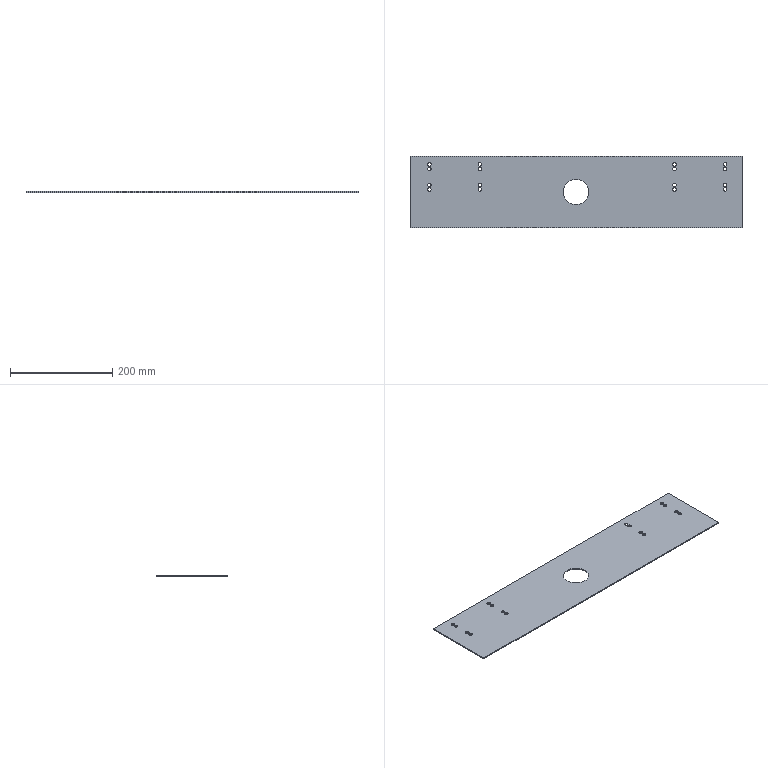Part | NX | 1 solid | 23 faces | box 650 x 140 x 2 mm | volume 176842 mm3 | cylinder 17 | plane 6 | commonest cylinder face diameters 7 x16 50 x1
STEP:
#1=CARTESIAN_POINT('',(325.,-70.,0.));
#2=VERTEX_POINT('',#1);
#3=CARTESIAN_POINT('',(325.,70.,0.));
#4=VERTEX_POINT('',#3);
#5=CARTESIAN_POINT('',(325.,-70.,0.));
#6=DIRECTION('',(0.,1.,0.));
#7=VECTOR('',#6,1000.);
#8=LINE('',#5,#7);
#9=EDGE_CURVE('',#2,#4,#8,.T.);
#10=ORIENTED_EDGE('',*,*,#9,.F.);
#11=CARTESIAN_POINT('',(325.,-70.,-2.));
#12=VERTEX_POINT('',#11);
#13=CARTESIAN_POINT('',(325.,-70.,-2.));
#14=DIRECTION('',(0.,0.,1.));
#15=VECTOR('',#14,1000.);
#16=LINE('',#13,#15);
#17=EDGE_CURVE('',#12,#2,#16,.T.);
#18=ORIENTED_EDGE('',*,*,#17,.F.);
#19=CARTESIAN_POINT('',(325.,70.,-2.));
#20=VERTEX_POINT('',#19);
#21=CARTESIAN_POINT('',(325.,-70.,-2.));
#22=DIRECTION('',(0.,1.,0.));
#23=VECTOR('',#22,1000.);
#24=LINE('',#21,#23);
#25=EDGE_CURVE('',#12,#20,#24,.T.);
#26=ORIENTED_EDGE('',*,*,#25,.T.);
#27=CARTESIAN_POINT('',(325.,70.,-2.));
#28=DIRECTION('',(0.,0.,1.));
#29=VECTOR('',#28,1000.);
#30=LINE('',#27,#29);
#31=EDGE_CURVE('',#20,#4,#30,.T.);
#32=ORIENTED_EDGE('',*,*,#31,.T.);
#33=EDGE_LOOP('',(#10,#18,#26,#32));
#34=FACE_BOUND('',#33,.T.);
#35=CARTESIAN_POINT('',(325.,-70.,-2.));
#36=DIRECTION('',(1.,0.,0.));
#37=DIRECTION('',(0.,0.,-1.));
#38=AXIS2_PLACEMENT_3D('',#35,#36,#37);
#39=PLANE('',#38);
#40=ADVANCED_FACE('',(#34),#39,.T.);
#41=CARTESIAN_POINT('',(-325.,-70.,0.));
#42=VERTEX_POINT('',#41);
#43=CARTESIAN_POINT('',(-325.,-70.,0.));
#44=DIRECTION('',(1.,0.,0.));
#45=VECTOR('',#44,1000.);
#46=LINE('',#43,#45);
#47=EDGE_CURVE('',#42,#2,#46,.T.);
#48=ORIENTED_EDGE('',*,*,#47,.F.);
#49=CARTESIAN_POINT('',(-325.,-70.,-2.));
#50=VERTEX_POINT('',#49);
#51=CARTESIAN_POINT('',(-325.,-70.,-2.));
#52=DIRECTION('',(0.,0.,1.));
#53=VECTOR('',#52,1000.);
#54=LINE('',#51,#53);
#55=EDGE_CURVE('',#50,#42,#54,.T.);
#56=ORIENTED_EDGE('',*,*,#55,.F.);
#57=CARTESIAN_POINT('',(-325.,-70.,-2.));
#58=DIRECTION('',(1.,0.,0.));
#59=VECTOR('',#58,1000.);
#60=LINE('',#57,#59);
#61=EDGE_CURVE('',#50,#12,#60,.T.);
#62=ORIENTED_EDGE('',*,*,#61,.T.);
#63=ORIENTED_EDGE('',*,*,#17,.T.);
#64=EDGE_LOOP('',(#48,#56,#62,#63));
#65=FACE_BOUND('',#64,.T.);
#66=CARTESIAN_POINT('',(-325.,-70.,-2.));
#67=DIRECTION('',(0.,-1.,0.));
#68=DIRECTION('',(0.,0.,-1.));
#69=AXIS2_PLACEMENT_3D('',#66,#67,#68);
#70=PLANE('',#69);
#71=ADVANCED_FACE('',(#65),#70,.T.);
#72=CARTESIAN_POINT('',(-325.,70.,0.));
#73=VERTEX_POINT('',#72);
#74=CARTESIAN_POINT('',(-325.,-70.,0.));
#75=DIRECTION('',(0.,-1.,0.));
#76=VECTOR('',#75,1000.);
#77=LINE('',#74,#76);
#78=EDGE_CURVE('',#73,#42,#77,.T.);
#79=ORIENTED_EDGE('',*,*,#78,.F.);
#80=CARTESIAN_POINT('',(-325.,70.,-2.));
#81=VERTEX_POINT('',#80);
#82=CARTESIAN_POINT('',(-325.,70.,-2.));
#83=DIRECTION('',(0.,0.,1.));
#84=VECTOR('',#83,1000.);
#85=LINE('',#82,#84);
#86=EDGE_CURVE('',#81,#73,#85,.T.);
#87=ORIENTED_EDGE('',*,*,#86,.F.);
#88=CARTESIAN_POINT('',(-325.,-70.,-2.));
#89=DIRECTION('',(0.,-1.,0.));
#90=VECTOR('',#89,1000.);
#91=LINE('',#88,#90);
#92=EDGE_CURVE('',#81,#50,#91,.T.);
#93=ORIENTED_EDGE('',*,*,#92,.T.);
#94=ORIENTED_EDGE('',*,*,#55,.T.);
#95=EDGE_LOOP('',(#79,#87,#93,#94));
#96=FACE_BOUND('',#95,.T.);
#97=CARTESIAN_POINT('',(-325.,-70.,-2.));
#98=DIRECTION('',(-1.,0.,0.));
#99=DIRECTION('',(0.,0.,1.));
#100=AXIS2_PLACEMENT_3D('',#97,#98,#99);
#101=PLANE('',#100);
#102=ADVANCED_FACE('',(#96),#101,.T.);
#103=CARTESIAN_POINT('',(-325.,70.,0.));
#104=DIRECTION('',(-1.,0.,0.));
#105=VECTOR('',#104,1000.);
#106=LINE('',#103,#105);
#107=EDGE_CURVE('',#4,#73,#106,.T.);
#108=ORIENTED_EDGE('',*,*,#107,.F.);
#109=ORIENTED_EDGE('',*,*,#31,.F.);
#110=CARTESIAN_POINT('',(-325.,70.,-2.));
#111=DIRECTION('',(-1.,0.,0.));
#112=VECTOR('',#111,1000.);
#113=LINE('',#110,#112);
#114=EDGE_CURVE('',#20,#81,#113,.T.);
#115=ORIENTED_EDGE('',*,*,#114,.T.);
#116=ORIENTED_EDGE('',*,*,#86,.T.);
#117=EDGE_LOOP('',(#108,#109,#115,#116));
#118=FACE_BOUND('',#117,.T.);
#119=CARTESIAN_POINT('',(-325.,70.,-2.));
#120=DIRECTION('',(0.,1.,0.));
#121=DIRECTION('',(0.,0.,1.));
#122=AXIS2_PLACEMENT_3D('',#119,#120,#121);
#123=PLANE('',#122);
#124=ADVANCED_FACE('',(#118),#123,.T.);
#125=CARTESIAN_POINT('',(-290.5,14.,-2.));
#126=VERTEX_POINT('',#125);
#127=CARTESIAN_POINT('',(-287.,14.,-2.));
#128=DIRECTION('',(0.,0.,-1.));
#129=DIRECTION('',(-1.,0.,0.));
#130=AXIS2_PLACEMENT_3D('',#127,#128,#129);
#131=CIRCLE('',#130,3.5);
#132=EDGE_CURVE('',#126,#126,#131,.T.);
#133=ORIENTED_EDGE('',*,*,#132,.F.);
#134=EDGE_LOOP('',(#133));
#135=FACE_BOUND('',#134,.T.);
#136=CARTESIAN_POINT('',(-191.5,14.,-2.));
#137=VERTEX_POINT('',#136);
#138=CARTESIAN_POINT('',(-188.,14.,-2.));
#139=DIRECTION('',(0.,0.,-1.));
#140=DIRECTION('',(-1.,0.,0.));
#141=AXIS2_PLACEMENT_3D('',#138,#139,#140);
#142=CIRCLE('',#141,3.5);
#143=EDGE_CURVE('',#137,#137,#142,.T.);
#144=ORIENTED_EDGE('',*,*,#143,.F.);
#145=EDGE_LOOP('',(#144));
#146=FACE_BOUND('',#145,.T.);
#147=CARTESIAN_POINT('',(-191.5,54.,-2.));
#148=VERTEX_POINT('',#147);
#149=CARTESIAN_POINT('',(-188.,54.,-2.));
#150=DIRECTION('',(0.,0.,-1.));
#151=DIRECTION('',(-1.,0.,0.));
#152=AXIS2_PLACEMENT_3D('',#149,#150,#151);
#153=CIRCLE('',#152,3.5);
#154=EDGE_CURVE('',#148,#148,#153,.T.);
#155=ORIENTED_EDGE('',*,*,#154,.F.);
#156=EDGE_LOOP('',(#155));
#157=FACE_BOUND('',#156,.T.);
#158=CARTESIAN_POINT('',(288.5,54.,-2.));
#159=VERTEX_POINT('',#158);
#160=CARTESIAN_POINT('',(292.,54.,-2.));
#161=DIRECTION('',(0.,0.,-1.));
#162=DIRECTION('',(-1.,0.,0.));
#163=AXIS2_PLACEMENT_3D('',#160,#161,#162);
#164=CIRCLE('',#163,3.5);
#165=EDGE_CURVE('',#159,#159,#164,.T.);
#166=ORIENTED_EDGE('',*,*,#165,.F.);
#167=EDGE_LOOP('',(#166));
#168=FACE_BOUND('',#167,.T.);
#169=CARTESIAN_POINT('',(288.5,14.,-2.));
#170=VERTEX_POINT('',#169);
#171=CARTESIAN_POINT('',(292.,14.,-2.));
#172=DIRECTION('',(0.,0.,-1.));
#173=DIRECTION('',(-1.,0.,0.));
#174=AXIS2_PLACEMENT_3D('',#171,#172,#173);
#175=CIRCLE('',#174,3.5);
#176=EDGE_CURVE('',#170,#170,#175,.T.);
#177=ORIENTED_EDGE('',*,*,#176,.F.);
#178=EDGE_LOOP('',(#177));
#179=FACE_BOUND('',#178,.T.);
#180=CARTESIAN_POINT('',(189.5,14.,-2.));
#181=VERTEX_POINT('',#180);
#182=CARTESIAN_POINT('',(193.,14.,-2.));
#183=DIRECTION('',(0.,0.,-1.));
#184=DIRECTION('',(-1.,0.,0.));
#185=AXIS2_PLACEMENT_3D('',#182,#183,#184);
#186=CIRCLE('',#185,3.5);
#187=EDGE_CURVE('',#181,#181,#186,.T.);
#188=ORIENTED_EDGE('',*,*,#187,.F.);
#189=EDGE_LOOP('',(#188));
#190=FACE_BOUND('',#189,.T.);
#191=CARTESIAN_POINT('',(189.5,54.,-2.));
#192=VERTEX_POINT('',#191);
#193=CARTESIAN_POINT('',(193.,54.,-2.));
#194=DIRECTION('',(0.,0.,-1.));
#195=DIRECTION('',(-1.,0.,0.));
#196=AXIS2_PLACEMENT_3D('',#193,#194,#195);
#197=CIRCLE('',#196,3.5);
#198=EDGE_CURVE('',#192,#192,#197,.T.);
#199=ORIENTED_EDGE('',*,*,#198,.F.);
#200=EDGE_LOOP('',(#199));
#201=FACE_BOUND('',#200,.T.);
#202=CARTESIAN_POINT('',(-290.5,54.,-2.));
#203=VERTEX_POINT('',#202);
#204=CARTESIAN_POINT('',(-287.,54.,-2.));
#205=DIRECTION('',(0.,0.,-1.));
#206=DIRECTION('',(-1.,0.,0.));
#207=AXIS2_PLACEMENT_3D('',#204,#205,#206);
#208=CIRCLE('',#207,3.5);
#209=EDGE_CURVE('',#203,#203,#208,.T.);
#210=ORIENTED_EDGE('',*,*,#209,.F.);
#211=EDGE_LOOP('',(#210));
#212=FACE_BOUND('',#211,.T.);
#213=CARTESIAN_POINT('',(-290.5,45.,-2.));
#214=VERTEX_POINT('',#213);
#215=CARTESIAN_POINT('',(-287.,45.,-2.));
#216=DIRECTION('',(0.,0.,-1.));
#217=DIRECTION('',(-1.,0.,0.));
#218=AXIS2_PLACEMENT_3D('',#215,#216,#217);
#219=CIRCLE('',#218,3.5);
#220=EDGE_CURVE('',#214,#214,#219,.T.);
#221=ORIENTED_EDGE('',*,*,#220,.F.);
#222=EDGE_LOOP('',(#221));
#223=FACE_BOUND('',#222,.T.);
#224=CARTESIAN_POINT('',(-290.5,5.,-2.));
#225=VERTEX_POINT('',#224);
#226=CARTESIAN_POINT('',(-287.,5.,-2.));
#227=DIRECTION('',(0.,0.,-1.));
#228=DIRECTION('',(-1.,0.,0.));
#229=AXIS2_PLACEMENT_3D('',#226,#227,#228);
#230=CIRCLE('',#229,3.5);
#231=EDGE_CURVE('',#225,#225,#230,.T.);
#232=ORIENTED_EDGE('',*,*,#231,.F.);
#233=EDGE_LOOP('',(#232));
#234=FACE_BOUND('',#233,.T.);
#235=CARTESIAN_POINT('',(-191.5,5.,-2.));
#236=VERTEX_POINT('',#235);
#237=CARTESIAN_POINT('',(-188.,5.,-2.));
#238=DIRECTION('',(0.,0.,-1.));
#239=DIRECTION('',(-1.,0.,0.));
#240=AXIS2_PLACEMENT_3D('',#237,#238,#239);
#241=CIRCLE('',#240,3.5);
#242=EDGE_CURVE('',#236,#236,#241,.T.);
#243=ORIENTED_EDGE('',*,*,#242,.F.);
#244=EDGE_LOOP('',(#243));
#245=FACE_BOUND('',#244,.T.);
#246=CARTESIAN_POINT('',(-191.5,45.,-2.));
#247=VERTEX_POINT('',#246);
#248=CARTESIAN_POINT('',(-188.,45.,-2.));
#249=DIRECTION('',(0.,0.,-1.));
#250=DIRECTION('',(-1.,0.,0.));
#251=AXIS2_PLACEMENT_3D('',#248,#249,#250);
#252=CIRCLE('',#251,3.5);
#253=EDGE_CURVE('',#247,#247,#252,.T.);
#254=ORIENTED_EDGE('',*,*,#253,.F.);
#255=EDGE_LOOP('',(#254));
#256=FACE_BOUND('',#255,.T.);
#257=CARTESIAN_POINT('',(288.5,45.,-2.));
#258=VERTEX_POINT('',#257);
#259=CARTESIAN_POINT('',(292.,45.,-2.));
#260=DIRECTION('',(0.,0.,-1.));
#261=DIRECTION('',(-1.,0.,0.));
#262=AXIS2_PLACEMENT_3D('',#259,#260,#261);
#263=CIRCLE('',#262,3.5);
#264=EDGE_CURVE('',#258,#258,#263,.T.);
#265=ORIENTED_EDGE('',*,*,#264,.F.);
#266=EDGE_LOOP('',(#265));
#267=FACE_BOUND('',#266,.T.);
#268=CARTESIAN_POINT('',(288.5,5.,-2.));
#269=VERTEX_POINT('',#268);
#270=CARTESIAN_POINT('',(292.,5.,-2.));
#271=DIRECTION('',(0.,0.,-1.));
#272=DIRECTION('',(-1.,0.,0.));
#273=AXIS2_PLACEMENT_3D('',#270,#271,#272);
#274=CIRCLE('',#273,3.5);
#275=EDGE_CURVE('',#269,#269,#274,.T.);
#276=ORIENTED_EDGE('',*,*,#275,.F.);
#277=EDGE_LOOP('',(#276));
#278=FACE_BOUND('',#277,.T.);
#279=CARTESIAN_POINT('',(189.5,5.,-2.));
#280=VERTEX_POINT('',#279);
#281=CARTESIAN_POINT('',(193.,5.,-2.));
#282=DIRECTION('',(0.,0.,-1.));
#283=DIRECTION('',(-1.,0.,0.));
#284=AXIS2_PLACEMENT_3D('',#281,#282,#283);
#285=CIRCLE('',#284,3.5);
#286=EDGE_CURVE('',#280,#280,#285,.T.);
#287=ORIENTED_EDGE('',*,*,#286,.F.);
#288=EDGE_LOOP('',(#287));
#289=FACE_BOUND('',#288,.T.);
#290=CARTESIAN_POINT('',(189.5,45.,-2.));
#291=VERTEX_POINT('',#290);
#292=CARTESIAN_POINT('',(193.,45.,-2.));
#293=DIRECTION('',(0.,0.,-1.));
#294=DIRECTION('',(-1.,0.,0.));
#295=AXIS2_PLACEMENT_3D('',#292,#293,#294);
#296=CIRCLE('',#295,3.5);
#297=EDGE_CURVE('',#291,#291,#296,.T.);
#298=ORIENTED_EDGE('',*,*,#297,.F.);
#299=EDGE_LOOP('',(#298));
#300=FACE_BOUND('',#299,.T.);
#301=CARTESIAN_POINT('',(-25.,0.,-2.));
#302=VERTEX_POINT('',#301);
#303=CARTESIAN_POINT('',(0.,0.,-2.));
#304=DIRECTION('',(0.,0.,-1.));
#305=DIRECTION('',(-1.,0.,0.));
#306=AXIS2_PLACEMENT_3D('',#303,#304,#305);
#307=CIRCLE('',#306,25.);
#308=EDGE_CURVE('',#302,#302,#307,.T.);
#309=ORIENTED_EDGE('',*,*,#308,.F.);
#310=EDGE_LOOP('',(#309));
#311=FACE_BOUND('',#310,.T.);
#312=ORIENTED_EDGE('',*,*,#25,.F.);
#313=ORIENTED_EDGE('',*,*,#61,.F.);
#314=ORIENTED_EDGE('',*,*,#92,.F.);
#315=ORIENTED_EDGE('',*,*,#114,.F.);
#316=EDGE_LOOP('',(#312,#313,#314,#315));
#317=FACE_BOUND('',#316,.T.);
#318=CARTESIAN_POINT('',(0.,0.,-2.));
#319=DIRECTION('',(0.,0.,-1.));
#320=DIRECTION('',(-1.,0.,0.));
#321=AXIS2_PLACEMENT_3D('',#318,#319,#320);
#322=PLANE('',#321);
#323=ADVANCED_FACE('',(#135,#146,#157,#168,#179,#190,#201,#212,#223,#234,#245,#256,#267,#278,#289,#300,#311,#317),#322,.T.);
#324=CARTESIAN_POINT('',(-283.5,14.,0.));
#325=VERTEX_POINT('',#324);
#326=CARTESIAN_POINT('',(-287.,14.,0.));
#327=DIRECTION('',(0.,0.,1.));
#328=DIRECTION('',(1.,0.,0.));
#329=AXIS2_PLACEMENT_3D('',#326,#327,#328);
#330=CIRCLE('',#329,3.5);
#331=EDGE_CURVE('',#325,#325,#330,.T.);
#332=ORIENTED_EDGE('',*,*,#331,.F.);
#333=EDGE_LOOP('',(#332));
#334=FACE_BOUND('',#333,.T.);
#335=CARTESIAN_POINT('',(-184.5,14.,0.));
#336=VERTEX_POINT('',#335);
#337=CARTESIAN_POINT('',(-188.,14.,0.));
#338=DIRECTION('',(0.,0.,1.));
#339=DIRECTION('',(1.,0.,0.));
#340=AXIS2_PLACEMENT_3D('',#337,#338,#339);
#341=CIRCLE('',#340,3.5);
#342=EDGE_CURVE('',#336,#336,#341,.T.);
#343=ORIENTED_EDGE('',*,*,#342,.F.);
#344=EDGE_LOOP('',(#343));
#345=FACE_BOUND('',#344,.T.);
#346=CARTESIAN_POINT('',(-184.5,54.,0.));
#347=VERTEX_POINT('',#346);
#348=CARTESIAN_POINT('',(-188.,54.,0.));
#349=DIRECTION('',(0.,0.,1.));
#350=DIRECTION('',(1.,0.,0.));
#351=AXIS2_PLACEMENT_3D('',#348,#349,#350);
#352=CIRCLE('',#351,3.5);
#353=EDGE_CURVE('',#347,#347,#352,.T.);
#354=ORIENTED_EDGE('',*,*,#353,.F.);
#355=EDGE_LOOP('',(#354));
#356=FACE_BOUND('',#355,.T.);
#357=CARTESIAN_POINT('',(295.5,54.,0.));
#358=VERTEX_POINT('',#357);
#359=CARTESIAN_POINT('',(292.,54.,0.));
#360=DIRECTION('',(0.,0.,1.));
#361=DIRECTION('',(1.,0.,0.));
#362=AXIS2_PLACEMENT_3D('',#359,#360,#361);
#363=CIRCLE('',#362,3.5);
#364=EDGE_CURVE('',#358,#358,#363,.T.);
#365=ORIENTED_EDGE('',*,*,#364,.F.);
#366=EDGE_LOOP('',(#365));
#367=FACE_BOUND('',#366,.T.);
#368=CARTESIAN_POINT('',(295.5,14.,0.));
#369=VERTEX_POINT('',#368);
#370=CARTESIAN_POINT('',(292.,14.,0.));
#371=DIRECTION('',(0.,0.,1.));
#372=DIRECTION('',(1.,0.,0.));
#373=AXIS2_PLACEMENT_3D('',#370,#371,#372);
#374=CIRCLE('',#373,3.5);
#375=EDGE_CURVE('',#369,#369,#374,.T.);
#376=ORIENTED_EDGE('',*,*,#375,.F.);
#377=EDGE_LOOP('',(#376));
#378=FACE_BOUND('',#377,.T.);
#379=CARTESIAN_POINT('',(196.5,14.,0.));
#380=VERTEX_POINT('',#379);
#381=CARTESIAN_POINT('',(193.,14.,0.));
#382=DIRECTION('',(0.,0.,1.));
#383=DIRECTION('',(1.,0.,0.));
#384=AXIS2_PLACEMENT_3D('',#381,#382,#383);
#385=CIRCLE('',#384,3.5);
#386=EDGE_CURVE('',#380,#380,#385,.T.);
#387=ORIENTED_EDGE('',*,*,#386,.F.);
#388=EDGE_LOOP('',(#387));
#389=FACE_BOUND('',#388,.T.);
#390=CARTESIAN_POINT('',(196.5,54.,0.));
#391=VERTEX_POINT('',#390);
#392=CARTESIAN_POINT('',(193.,54.,0.));
#393=DIRECTION('',(0.,0.,1.));
#394=DIRECTION('',(1.,0.,0.));
#395=AXIS2_PLACEMENT_3D('',#392,#393,#394);
#396=CIRCLE('',#395,3.5);
#397=EDGE_CURVE('',#391,#391,#396,.T.);
#398=ORIENTED_EDGE('',*,*,#397,.F.);
#399=EDGE_LOOP('',(#398));
#400=FACE_BOUND('',#399,.T.);
#401=CARTESIAN_POINT('',(-283.5,54.,0.));
#402=VERTEX_POINT('',#401);
#403=CARTESIAN_POINT('',(-287.,54.,0.));
#404=DIRECTION('',(0.,0.,1.));
#405=DIRECTION('',(1.,0.,0.));
#406=AXIS2_PLACEMENT_3D('',#403,#404,#405);
#407=CIRCLE('',#406,3.5);
#408=EDGE_CURVE('',#402,#402,#407,.T.);
#409=ORIENTED_EDGE('',*,*,#408,.F.);
#410=EDGE_LOOP('',(#409));
#411=FACE_BOUND('',#410,.T.);
#412=CARTESIAN_POINT('',(-283.5,45.,0.));
#413=VERTEX_POINT('',#412);
#414=CARTESIAN_POINT('',(-287.,45.,0.));
#415=DIRECTION('',(0.,0.,1.));
#416=DIRECTION('',(1.,0.,0.));
#417=AXIS2_PLACEMENT_3D('',#414,#415,#416);
#418=CIRCLE('',#417,3.5);
#419=EDGE_CURVE('',#413,#413,#418,.T.);
#420=ORIENTED_EDGE('',*,*,#419,.F.);
#421=EDGE_LOOP('',(#420));
#422=FACE_BOUND('',#421,.T.);
#423=CARTESIAN_POINT('',(-283.5,5.,0.));
#424=VERTEX_POINT('',#423);
#425=CARTESIAN_POINT('',(-287.,5.,0.));
#426=DIRECTION('',(0.,0.,1.));
#427=DIRECTION('',(1.,0.,0.));
#428=AXIS2_PLACEMENT_3D('',#425,#426,#427);
#429=CIRCLE('',#428,3.5);
#430=EDGE_CURVE('',#424,#424,#429,.T.);
#431=ORIENTED_EDGE('',*,*,#430,.F.);
#432=EDGE_LOOP('',(#431));
#433=FACE_BOUND('',#432,.T.);
#434=CARTESIAN_POINT('',(-184.5,5.,0.));
#435=VERTEX_POINT('',#434);
#436=CARTESIAN_POINT('',(-188.,5.,0.));
#437=DIRECTION('',(0.,0.,1.));
#438=DIRECTION('',(1.,0.,0.));
#439=AXIS2_PLACEMENT_3D('',#436,#437,#438);
#440=CIRCLE('',#439,3.5);
#441=EDGE_CURVE('',#435,#435,#440,.T.);
#442=ORIENTED_EDGE('',*,*,#441,.F.);
#443=EDGE_LOOP('',(#442));
#444=FACE_BOUND('',#443,.T.);
#445=CARTESIAN_POINT('',(-184.5,45.,0.));
#446=VERTEX_POINT('',#445);
#447=CARTESIAN_POINT('',(-188.,45.,0.));
#448=DIRECTION('',(0.,0.,1.));
#449=DIRECTION('',(1.,0.,0.));
#450=AXIS2_PLACEMENT_3D('',#447,#448,#449);
#451=CIRCLE('',#450,3.5);
#452=EDGE_CURVE('',#446,#446,#451,.T.);
#453=ORIENTED_EDGE('',*,*,#452,.F.);
#454=EDGE_LOOP('',(#453));
#455=FACE_BOUND('',#454,.T.);
#456=CARTESIAN_POINT('',(295.5,45.,0.));
#457=VERTEX_POINT('',#456);
#458=CARTESIAN_POINT('',(292.,45.,0.));
#459=DIRECTION('',(0.,0.,1.));
#460=DIRECTION('',(1.,0.,0.));
#461=AXIS2_PLACEMENT_3D('',#458,#459,#460);
#462=CIRCLE('',#461,3.5);
#463=EDGE_CURVE('',#457,#457,#462,.T.);
#464=ORIENTED_EDGE('',*,*,#463,.F.);
#465=EDGE_LOOP('',(#464));
#466=FACE_BOUND('',#465,.T.);
#467=CARTESIAN_POINT('',(295.5,5.,0.));
#468=VERTEX_POINT('',#467);
#469=CARTESIAN_POINT('',(292.,5.,0.));
#470=DIRECTION('',(0.,0.,1.));
#471=DIRECTION('',(1.,0.,0.));
#472=AXIS2_PLACEMENT_3D('',#469,#470,#471);
#473=CIRCLE('',#472,3.5);
#474=EDGE_CURVE('',#468,#468,#473,.T.);
#475=ORIENTED_EDGE('',*,*,#474,.F.);
#476=EDGE_LOOP('',(#475));
#477=FACE_BOUND('',#476,.T.);
#478=CARTESIAN_POINT('',(196.5,5.,0.));
#479=VERTEX_POINT('',#478);
#480=CARTESIAN_POINT('',(193.,5.,0.));
#481=DIRECTION('',(0.,0.,1.));
#482=DIRECTION('',(1.,0.,0.));
#483=AXIS2_PLACEMENT_3D('',#480,#481,#482);
#484=CIRCLE('',#483,3.5);
#485=EDGE_CURVE('',#479,#479,#484,.T.);
#486=ORIENTED_EDGE('',*,*,#485,.F.);
#487=EDGE_LOOP('',(#486));
#488=FACE_BOUND('',#487,.T.);
#489=CARTESIAN_POINT('',(196.5,45.,0.));
#490=VERTEX_POINT('',#489);
#491=CARTESIAN_POINT('',(193.,45.,0.));
#492=DIRECTION('',(0.,0.,1.));
#493=DIRECTION('',(1.,0.,0.));
#494=AXIS2_PLACEMENT_3D('',#491,#492,#493);
#495=CIRCLE('',#494,3.5);
#496=EDGE_CURVE('',#490,#490,#495,.T.);
#497=ORIENTED_EDGE('',*,*,#496,.F.);
#498=EDGE_LOOP('',(#497));
#499=FACE_BOUND('',#498,.T.);
#500=CARTESIAN_POINT('',(25.,0.,0.));
#501=VERTEX_POINT('',#500);
#502=CARTESIAN_POINT('',(0.,0.,0.));
#503=DIRECTION('',(0.,0.,1.));
#504=DIRECTION('',(1.,0.,0.));
#505=AXIS2_PLACEMENT_3D('',#502,#503,#504);
#506=CIRCLE('',#505,25.);
#507=EDGE_CURVE('',#501,#501,#506,.T.);
#508=ORIENTED_EDGE('',*,*,#507,.F.);
#509=EDGE_LOOP('',(#508));
#510=FACE_BOUND('',#509,.T.);
#511=ORIENTED_EDGE('',*,*,#9,.T.);
#512=ORIENTED_EDGE('',*,*,#107,.T.);
#513=ORIENTED_EDGE('',*,*,#78,.T.);
#514=ORIENTED_EDGE('',*,*,#47,.T.);
#515=EDGE_LOOP('',(#511,#512,#513,#514));
#516=FACE_BOUND('',#515,.T.);
#517=CARTESIAN_POINT('',(0.,0.,0.));
#518=DIRECTION('',(0.,0.,-1.));
#519=DIRECTION('',(-1.,0.,0.));
#520=AXIS2_PLACEMENT_3D('',#517,#518,#519);
#521=PLANE('',#520);
#522=ADVANCED_FACE('',(#334,#345,#356,#367,#378,#389,#400,#411,#422,#433,#444,#455,#466,#477,#488,#499,#510,#516),#521,.F.);
#523=ORIENTED_EDGE('',*,*,#308,.T.);
#524=EDGE_LOOP('',(#523));
#525=FACE_BOUND('',#524,.T.);
#526=ORIENTED_EDGE('',*,*,#507,.T.);
#527=EDGE_LOOP('',(#526));
#528=FACE_BOUND('',#527,.T.);
#529=CARTESIAN_POINT('',(0.,0.,-10.));
#530=DIRECTION('',(0.,0.,1.));
#531=DIRECTION('',(1.,0.,0.));
#532=AXIS2_PLACEMENT_3D('',#529,#530,#531);
#533=CYLINDRICAL_SURFACE('',#532,25.);
#534=ADVANCED_FACE('',(#525,#528),#533,.F.);
#535=ORIENTED_EDGE('',*,*,#297,.T.);
#536=EDGE_LOOP('',(#535));
#537=FACE_BOUND('',#536,.T.);
#538=ORIENTED_EDGE('',*,*,#496,.T.);
#539=EDGE_LOOP('',(#538));
#540=FACE_BOUND('',#539,.T.);
#541=CARTESIAN_POINT('',(193.,45.,0.));
#542=DIRECTION('',(0.,0.,1.));
#543=DIRECTION('',(1.,0.,0.));
#544=AXIS2_PLACEMENT_3D('',#541,#542,#543);
#545=CYLINDRICAL_SURFACE('',#544,3.5);
#546=ADVANCED_FACE('',(#537,#540),#545,.F.);
#547=ORIENTED_EDGE('',*,*,#286,.T.);
#548=EDGE_LOOP('',(#547));
#549=FACE_BOUND('',#548,.T.);
#550=ORIENTED_EDGE('',*,*,#485,.T.);
#551=EDGE_LOOP('',(#550));
#552=FACE_BOUND('',#551,.T.);
#553=CARTESIAN_POINT('',(193.,5.,0.));
#554=DIRECTION('',(0.,0.,1.));
#555=DIRECTION('',(1.,0.,0.));
#556=AXIS2_PLACEMENT_3D('',#553,#554,#555);
#557=CYLINDRICAL_SURFACE('',#556,3.5);
#558=ADVANCED_FACE('',(#549,#552),#557,.F.);
#559=ORIENTED_EDGE('',*,*,#275,.T.);
#560=EDGE_LOOP('',(#559));
#561=FACE_BOUND('',#560,.T.);
#562=ORIENTED_EDGE('',*,*,#474,.T.);
#563=EDGE_LOOP('',(#562));
#564=FACE_BOUND('',#563,.T.);
#565=CARTESIAN_POINT('',(292.,5.,0.));
#566=DIRECTION('',(0.,0.,1.));
#567=DIRECTION('',(1.,0.,0.));
#568=AXIS2_PLACEMENT_3D('',#565,#566,#567);
#569=CYLINDRICAL_SURFACE('',#568,3.5);
#570=ADVANCED_FACE('',(#561,#564),#569,.F.);
#571=ORIENTED_EDGE('',*,*,#264,.T.);
#572=EDGE_LOOP('',(#571));
#573=FACE_BOUND('',#572,.T.);
#574=ORIENTED_EDGE('',*,*,#463,.T.);
#575=EDGE_LOOP('',(#574));
#576=FACE_BOUND('',#575,.T.);
#577=CARTESIAN_POINT('',(292.,45.,0.));
#578=DIRECTION('',(0.,0.,1.));
#579=DIRECTION('',(1.,0.,0.));
#580=AXIS2_PLACEMENT_3D('',#577,#578,#579);
#581=CYLINDRICAL_SURFACE('',#580,3.5);
#582=ADVANCED_FACE('',(#573,#576),#581,.F.);
#583=ORIENTED_EDGE('',*,*,#253,.T.);
#584=EDGE_LOOP('',(#583));
#585=FACE_BOUND('',#584,.T.);
#586=ORIENTED_EDGE('',*,*,#452,.T.);
#587=EDGE_LOOP('',(#586));
#588=FACE_BOUND('',#587,.T.);
#589=CARTESIAN_POINT('',(-188.,45.,0.));
#590=DIRECTION('',(0.,0.,1.));
#591=DIRECTION('',(1.,0.,0.));
#592=AXIS2_PLACEMENT_3D('',#589,#590,#591);
#593=CYLINDRICAL_SURFACE('',#592,3.5);
#594=ADVANCED_FACE('',(#585,#588),#593,.F.);
#595=ORIENTED_EDGE('',*,*,#242,.T.);
#596=EDGE_LOOP('',(#595));
#597=FACE_BOUND('',#596,.T.);
#598=ORIENTED_EDGE('',*,*,#441,.T.);
#599=EDGE_LOOP('',(#598));
#600=FACE_BOUND('',#599,.T.);
#601=CARTESIAN_POINT('',(-188.,5.,0.));
#602=DIRECTION('',(0.,0.,1.));
#603=DIRECTION('',(1.,0.,0.));
#604=AXIS2_PLACEMENT_3D('',#601,#602,#603);
#605=CYLINDRICAL_SURFACE('',#604,3.5);
#606=ADVANCED_FACE('',(#597,#600),#605,.F.);
#607=ORIENTED_EDGE('',*,*,#231,.T.);
#608=EDGE_LOOP('',(#607));
#609=FACE_BOUND('',#608,.T.);
#610=ORIENTED_EDGE('',*,*,#430,.T.);
#611=EDGE_LOOP('',(#610));
#612=FACE_BOUND('',#611,.T.);
#613=CARTESIAN_POINT('',(-287.,5.,0.));
#614=DIRECTION('',(0.,0.,1.));
#615=DIRECTION('',(1.,0.,0.));
#616=AXIS2_PLACEMENT_3D('',#613,#614,#615);
#617=CYLINDRICAL_SURFACE('',#616,3.5);
#618=ADVANCED_FACE('',(#609,#612),#617,.F.);
#619=ORIENTED_EDGE('',*,*,#220,.T.);
#620=EDGE_LOOP('',(#619));
#621=FACE_BOUND('',#620,.T.);
#622=ORIENTED_EDGE('',*,*,#419,.T.);
#623=EDGE_LOOP('',(#622));
#624=FACE_BOUND('',#623,.T.);
#625=CARTESIAN_POINT('',(-287.,45.,0.));
#626=DIRECTION('',(0.,0.,1.));
#627=DIRECTION('',(1.,0.,0.));
#628=AXIS2_PLACEMENT_3D('',#625,#626,#627);
#629=CYLINDRICAL_SURFACE('',#628,3.5);
#630=ADVANCED_FACE('',(#621,#624),#629,.F.);
#631=ORIENTED_EDGE('',*,*,#209,.T.);
#632=EDGE_LOOP('',(#631));
#633=FACE_BOUND('',#632,.T.);
#634=ORIENTED_EDGE('',*,*,#408,.T.);
#635=EDGE_LOOP('',(#634));
#636=FACE_BOUND('',#635,.T.);
#637=CARTESIAN_POINT('',(-287.,54.,0.));
#638=DIRECTION('',(0.,0.,1.));
#639=DIRECTION('',(1.,0.,0.));
#640=AXIS2_PLACEMENT_3D('',#637,#638,#639);
#641=CYLINDRICAL_SURFACE('',#640,3.5);
#642=ADVANCED_FACE('',(#633,#636),#641,.F.);
#643=ORIENTED_EDGE('',*,*,#198,.T.);
#644=EDGE_LOOP('',(#643));
#645=FACE_BOUND('',#644,.T.);
#646=ORIENTED_EDGE('',*,*,#397,.T.);
#647=EDGE_LOOP('',(#646));
#648=FACE_BOUND('',#647,.T.);
#649=CARTESIAN_POINT('',(193.,54.,0.));
#650=DIRECTION('',(0.,0.,1.));
#651=DIRECTION('',(1.,0.,0.));
#652=AXIS2_PLACEMENT_3D('',#649,#650,#651);
#653=CYLINDRICAL_SURFACE('',#652,3.5);
#654=ADVANCED_FACE('',(#645,#648),#653,.F.);
#655=ORIENTED_EDGE('',*,*,#187,.T.);
#656=EDGE_LOOP('',(#655));
#657=FACE_BOUND('',#656,.T.);
#658=ORIENTED_EDGE('',*,*,#386,.T.);
#659=EDGE_LOOP('',(#658));
#660=FACE_BOUND('',#659,.T.);
#661=CARTESIAN_POINT('',(193.,14.,0.));
#662=DIRECTION('',(0.,0.,1.));
#663=DIRECTION('',(1.,0.,0.));
#664=AXIS2_PLACEMENT_3D('',#661,#662,#663);
#665=CYLINDRICAL_SURFACE('',#664,3.5);
#666=ADVANCED_FACE('',(#657,#660),#665,.F.);
#667=ORIENTED_EDGE('',*,*,#176,.T.);
#668=EDGE_LOOP('',(#667));
#669=FACE_BOUND('',#668,.T.);
#670=ORIENTED_EDGE('',*,*,#375,.T.);
#671=EDGE_LOOP('',(#670));
#672=FACE_BOUND('',#671,.T.);
#673=CARTESIAN_POINT('',(292.,14.,0.));
#674=DIRECTION('',(0.,0.,1.));
#675=DIRECTION('',(1.,0.,0.));
#676=AXIS2_PLACEMENT_3D('',#673,#674,#675);
#677=CYLINDRICAL_SURFACE('',#676,3.5);
#678=ADVANCED_FACE('',(#669,#672),#677,.F.);
#679=ORIENTED_EDGE('',*,*,#165,.T.);
#680=EDGE_LOOP('',(#679));
#681=FACE_BOUND('',#680,.T.);
#682=ORIENTED_EDGE('',*,*,#364,.T.);
#683=EDGE_LOOP('',(#682));
#684=FACE_BOUND('',#683,.T.);
#685=CARTESIAN_POINT('',(292.,54.,0.));
#686=DIRECTION('',(0.,0.,1.));
#687=DIRECTION('',(1.,0.,0.));
#688=AXIS2_PLACEMENT_3D('',#685,#686,#687);
#689=CYLINDRICAL_SURFACE('',#688,3.5);
#690=ADVANCED_FACE('',(#681,#684),#689,.F.);
#691=ORIENTED_EDGE('',*,*,#154,.T.);
#692=EDGE_LOOP('',(#691));
#693=FACE_BOUND('',#692,.T.);
#694=ORIENTED_EDGE('',*,*,#353,.T.);
#695=EDGE_LOOP('',(#694));
#696=FACE_BOUND('',#695,.T.);
#697=CARTESIAN_POINT('',(-188.,54.,0.));
#698=DIRECTION('',(0.,0.,1.));
#699=DIRECTION('',(1.,0.,0.));
#700=AXIS2_PLACEMENT_3D('',#697,#698,#699);
#701=CYLINDRICAL_SURFACE('',#700,3.5);
#702=ADVANCED_FACE('',(#693,#696),#701,.F.);
#703=ORIENTED_EDGE('',*,*,#143,.T.);
#704=EDGE_LOOP('',(#703));
#705=FACE_BOUND('',#704,.T.);
#706=ORIENTED_EDGE('',*,*,#342,.T.);
#707=EDGE_LOOP('',(#706));
#708=FACE_BOUND('',#707,.T.);
#709=CARTESIAN_POINT('',(-188.,14.,0.));
#710=DIRECTION('',(0.,0.,1.));
#711=DIRECTION('',(1.,0.,0.));
#712=AXIS2_PLACEMENT_3D('',#709,#710,#711);
#713=CYLINDRICAL_SURFACE('',#712,3.5);
#714=ADVANCED_FACE('',(#705,#708),#713,.F.);
#715=ORIENTED_EDGE('',*,*,#132,.T.);
#716=EDGE_LOOP('',(#715));
#717=FACE_BOUND('',#716,.T.);
#718=ORIENTED_EDGE('',*,*,#331,.T.);
#719=EDGE_LOOP('',(#718));
#720=FACE_BOUND('',#719,.T.);
#721=CARTESIAN_POINT('',(-287.,14.,0.));
#722=DIRECTION('',(0.,0.,1.));
#723=DIRECTION('',(1.,0.,0.));
#724=AXIS2_PLACEMENT_3D('',#721,#722,#723);
#725=CYLINDRICAL_SURFACE('',#724,3.5);
#726=ADVANCED_FACE('',(#717,#720),#725,.F.);
#727=CLOSED_SHELL('',(#40,#71,#102,#124,#323,#522,#534,#546,#558,#570,#582,#594,#606,#618,#630,#642,#654,#666,#678,#690,#702,#714,#726));
#728=MANIFOLD_SOLID_BREP('',#727);
#729=(LENGTH_UNIT()NAMED_UNIT(*)SI_UNIT(.MILLI.,.METRE.));
#730=UNCERTAINTY_MEASURE_WITH_UNIT(LENGTH_MEASURE(0.00001),#729,'','');
#731=(NAMED_UNIT(*)PLANE_ANGLE_UNIT()SI_UNIT($,.RADIAN.));
#732=(NAMED_UNIT(*)SI_UNIT($,.STERADIAN.)SOLID_ANGLE_UNIT());
#733=(GEOMETRIC_REPRESENTATION_CONTEXT(3)GLOBAL_UNCERTAINTY_ASSIGNED_CONTEXT((#730))GLOBAL_UNIT_ASSIGNED_CONTEXT((#729,#731,#732))REPRESENTATION_CONTEXT('',''));
#734=ADVANCED_BREP_SHAPE_REPRESENTATION('',(#728),#733);